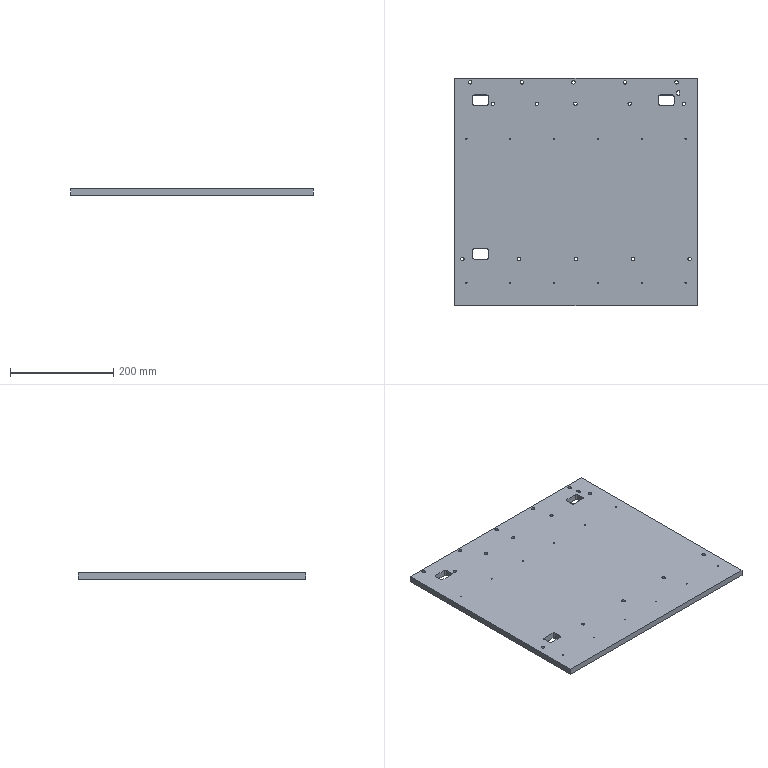Part | NX | features BREP 1 | 1 solid | 194 faces | box 470 x 440 x 12 mm | volume 2442341 mm3 | cylinder 116 | cone 40 | plane 38 | commonest cylinder face diameters 2.5 x40 6.6 x30 13 x20 6 x12 12 x10 4.5 x2